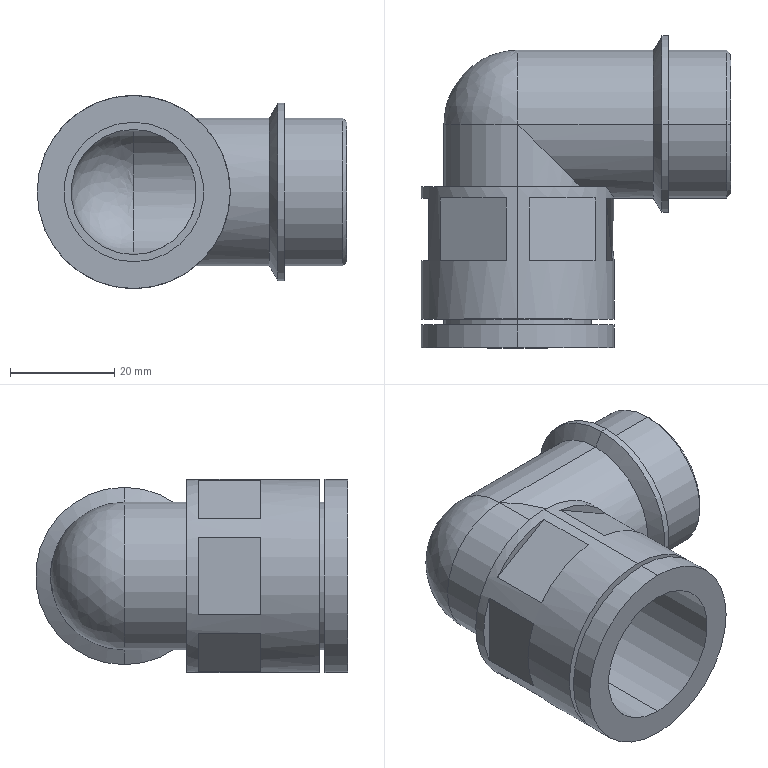Part | STEP file | 00177577_EZT_L-SCH.SCHL.VER._MKRL-23-PG-21.1 | 1 solid | 52 faces | box 59.35 x 59.85 x 37 mm | volume 23850 mm3 | plane 25 | cylinder 21 | cone 4 | spline 2 | commonest cylinder face diameters 28.3 x9 24 x4 37 x4 26.78 x2 34 x2